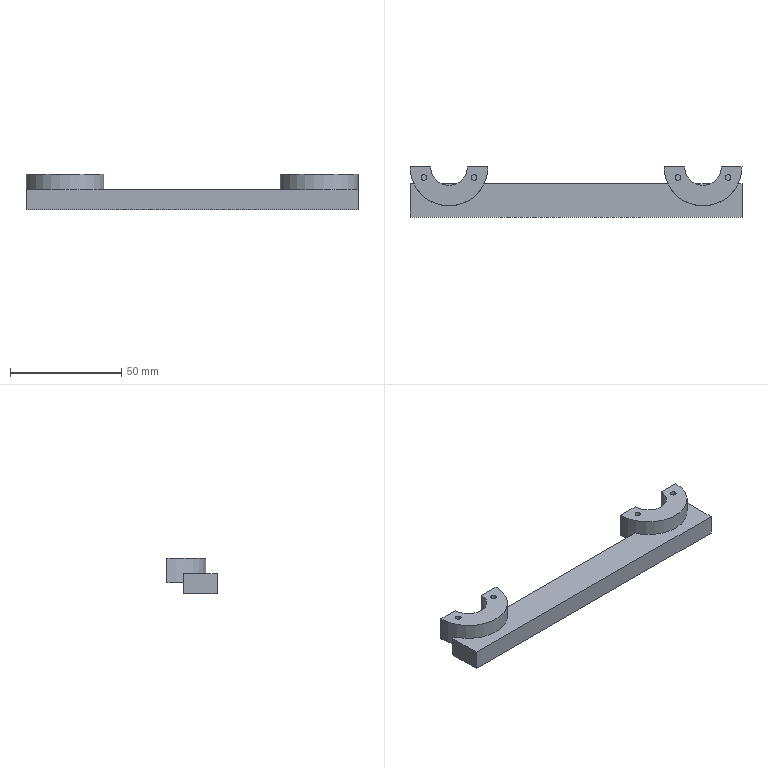Part | NX | 3 solids | 30 faces | box 149 x 22.5 x 16 mm | volume 26416 mm3 | plane 20 | cylinder 10 | commonest cylinder face diameters 2.5 x4 35 x4 16.5 x2
STEP:
#1=CARTESIAN_POINT('',(-53.811,-7.5,-7.));
#2=VERTEX_POINT('',#1);
#3=CARTESIAN_POINT('',(-22.189,-7.5,-7.));
#4=VERTEX_POINT('',#3);
#5=CARTESIAN_POINT('',(-38.,0.,-7.));
#6=DIRECTION('',(0.,0.,1.));
#7=DIRECTION('',(1.,0.,0.));
#8=AXIS2_PLACEMENT_3D('',#5,#6,#7);
#9=CIRCLE('',#8,17.5);
#10=EDGE_CURVE('',#2,#4,#9,.T.);
#11=ORIENTED_EDGE('',*,*,#10,.F.);
#12=CARTESIAN_POINT('',(-136.189,-7.5,-7.));
#13=VERTEX_POINT('',#12);
#14=CARTESIAN_POINT('',(-95.,-7.5,-7.));
#15=DIRECTION('',(1.,0.,0.));
#16=VECTOR('',#15,1000.);
#17=LINE('',#14,#16);
#18=EDGE_CURVE('',#13,#2,#17,.T.);
#19=ORIENTED_EDGE('',*,*,#18,.F.);
#20=CARTESIAN_POINT('',(-167.811,-7.5,-7.));
#21=VERTEX_POINT('',#20);
#22=CARTESIAN_POINT('',(-152.,0.,-7.));
#23=DIRECTION('',(0.,0.,1.));
#24=DIRECTION('',(1.,0.,0.));
#25=AXIS2_PLACEMENT_3D('',#22,#23,#24);
#26=CIRCLE('',#25,17.5);
#27=EDGE_CURVE('',#21,#13,#26,.T.);
#28=ORIENTED_EDGE('',*,*,#27,.F.);
#29=CARTESIAN_POINT('',(-169.5,-7.5,-7.));
#30=VERTEX_POINT('',#29);
#31=CARTESIAN_POINT('',(-95.,-7.5,-7.));
#32=DIRECTION('',(1.,0.,0.));
#33=VECTOR('',#32,1000.);
#34=LINE('',#31,#33);
#35=EDGE_CURVE('',#30,#21,#34,.T.);
#36=ORIENTED_EDGE('',*,*,#35,.F.);
#37=CARTESIAN_POINT('',(-169.5,-22.5,-7.));
#38=VERTEX_POINT('',#37);
#39=CARTESIAN_POINT('',(-169.5,-8.75,-7.));
#40=DIRECTION('',(0.,1.,0.));
#41=VECTOR('',#40,1000.);
#42=LINE('',#39,#41);
#43=EDGE_CURVE('',#38,#30,#42,.T.);
#44=ORIENTED_EDGE('',*,*,#43,.F.);
#45=CARTESIAN_POINT('',(-20.5,-22.5,-7.));
#46=VERTEX_POINT('',#45);
#47=CARTESIAN_POINT('',(-95.,-22.5,-7.));
#48=DIRECTION('',(-1.,0.,0.));
#49=VECTOR('',#48,1000.);
#50=LINE('',#47,#49);
#51=EDGE_CURVE('',#46,#38,#50,.T.);
#52=ORIENTED_EDGE('',*,*,#51,.F.);
#53=CARTESIAN_POINT('',(-20.5,-7.5,-7.));
#54=VERTEX_POINT('',#53);
#55=CARTESIAN_POINT('',(-20.5,-8.75,-7.));
#56=DIRECTION('',(0.,-1.,0.));
#57=VECTOR('',#56,1000.);
#58=LINE('',#55,#57);
#59=EDGE_CURVE('',#54,#46,#58,.T.);
#60=ORIENTED_EDGE('',*,*,#59,.F.);
#61=CARTESIAN_POINT('',(-95.,-7.5,-7.));
#62=DIRECTION('',(1.,0.,0.));
#63=VECTOR('',#62,1000.);
#64=LINE('',#61,#63);
#65=EDGE_CURVE('',#4,#54,#64,.T.);
#66=ORIENTED_EDGE('',*,*,#65,.F.);
#67=EDGE_LOOP('',(#11,#19,#28,#36,#44,#52,#60,#66));
#68=FACE_BOUND('',#67,.T.);
#69=CARTESIAN_POINT('',(-95.,-8.75,-7.));
#70=DIRECTION('',(0.,0.,1.));
#71=DIRECTION('',(1.,0.,0.));
#72=AXIS2_PLACEMENT_3D('',#69,#70,#71);
#73=PLANE('',#72);
#74=ADVANCED_FACE('',(#68),#73,.T.);
#75=CARTESIAN_POINT('',(-53.811,-7.5,-11.));
#76=VERTEX_POINT('',#75);
#77=CARTESIAN_POINT('',(-22.189,-7.5,-11.));
#78=VERTEX_POINT('',#77);
#79=CARTESIAN_POINT('',(-95.,-7.5,-11.));
#80=DIRECTION('',(1.,0.,0.));
#81=VECTOR('',#80,1000.);
#82=LINE('',#79,#81);
#83=EDGE_CURVE('',#76,#78,#82,.T.);
#84=ORIENTED_EDGE('',*,*,#83,.F.);
#85=CARTESIAN_POINT('',(-38.,0.,-11.));
#86=DIRECTION('',(0.,0.,1.));
#87=DIRECTION('',(1.,0.,0.));
#88=AXIS2_PLACEMENT_3D('',#85,#86,#87);
#89=CIRCLE('',#88,17.5);
#90=EDGE_CURVE('',#78,#76,#89,.F.);
#91=ORIENTED_EDGE('',*,*,#90,.F.);
#92=EDGE_LOOP('',(#84,#91));
#93=FACE_BOUND('',#92,.T.);
#94=CARTESIAN_POINT('',(-38.,0.,-11.));
#95=DIRECTION('',(0.,0.,1.));
#96=DIRECTION('',(1.,0.,0.));
#97=AXIS2_PLACEMENT_3D('',#94,#95,#96);
#98=PLANE('',#97);
#99=ADVANCED_FACE('',(#93),#98,.T.);
#100=CARTESIAN_POINT('',(-167.811,-7.5,-11.));
#101=VERTEX_POINT('',#100);
#102=CARTESIAN_POINT('',(-136.189,-7.5,-11.));
#103=VERTEX_POINT('',#102);
#104=CARTESIAN_POINT('',(-95.,-7.5,-11.));
#105=DIRECTION('',(1.,0.,0.));
#106=VECTOR('',#105,1000.);
#107=LINE('',#104,#106);
#108=EDGE_CURVE('',#101,#103,#107,.T.);
#109=ORIENTED_EDGE('',*,*,#108,.F.);
#110=CARTESIAN_POINT('',(-152.,0.,-11.));
#111=DIRECTION('',(0.,0.,1.));
#112=DIRECTION('',(1.,0.,0.));
#113=AXIS2_PLACEMENT_3D('',#110,#111,#112);
#114=CIRCLE('',#113,17.5);
#115=EDGE_CURVE('',#103,#101,#114,.F.);
#116=ORIENTED_EDGE('',*,*,#115,.F.);
#117=EDGE_LOOP('',(#109,#116));
#118=FACE_BOUND('',#117,.T.);
#119=CARTESIAN_POINT('',(-152.,0.,-11.));
#120=DIRECTION('',(0.,0.,1.));
#121=DIRECTION('',(1.,0.,0.));
#122=AXIS2_PLACEMENT_3D('',#119,#120,#121);
#123=PLANE('',#122);
#124=ADVANCED_FACE('',(#118),#123,.T.);
#125=CARTESIAN_POINT('',(-20.5,-22.5,-16.));
#126=VERTEX_POINT('',#125);
#127=CARTESIAN_POINT('',(-20.5,-22.5,-11.));
#128=DIRECTION('',(0.,0.,1.));
#129=VECTOR('',#128,1000.);
#130=LINE('',#127,#129);
#131=EDGE_CURVE('',#126,#46,#130,.T.);
#132=ORIENTED_EDGE('',*,*,#131,.T.);
#133=ORIENTED_EDGE('',*,*,#51,.T.);
#134=CARTESIAN_POINT('',(-169.5,-22.5,-16.));
#135=VERTEX_POINT('',#134);
#136=CARTESIAN_POINT('',(-169.5,-22.5,-11.));
#137=DIRECTION('',(0.,0.,1.));
#138=VECTOR('',#137,1000.);
#139=LINE('',#136,#138);
#140=EDGE_CURVE('',#135,#38,#139,.T.);
#141=ORIENTED_EDGE('',*,*,#140,.F.);
#142=CARTESIAN_POINT('',(-95.,-22.5,-16.));
#143=DIRECTION('',(1.,0.,0.));
#144=VECTOR('',#143,1000.);
#145=LINE('',#142,#144);
#146=EDGE_CURVE('',#135,#126,#145,.T.);
#147=ORIENTED_EDGE('',*,*,#146,.T.);
#148=EDGE_LOOP('',(#132,#133,#141,#147));
#149=FACE_BOUND('',#148,.T.);
#150=CARTESIAN_POINT('',(-95.,-22.5,-11.));
#151=DIRECTION('',(0.,-1.,0.));
#152=DIRECTION('',(0.,0.,-1.));
#153=AXIS2_PLACEMENT_3D('',#150,#151,#152);
#154=PLANE('',#153);
#155=ADVANCED_FACE('',(#149),#154,.T.);
#156=ORIENTED_EDGE('',*,*,#140,.T.);
#157=ORIENTED_EDGE('',*,*,#43,.T.);
#158=CARTESIAN_POINT('',(-169.5,-7.5,-16.));
#159=VERTEX_POINT('',#158);
#160=CARTESIAN_POINT('',(-169.5,-7.5,-11.));
#161=DIRECTION('',(0.,0.,1.));
#162=VECTOR('',#161,1000.);
#163=LINE('',#160,#162);
#164=EDGE_CURVE('',#159,#30,#163,.T.);
#165=ORIENTED_EDGE('',*,*,#164,.F.);
#166=CARTESIAN_POINT('',(-169.5,-8.75,-16.));
#167=DIRECTION('',(0.,-1.,0.));
#168=VECTOR('',#167,1000.);
#169=LINE('',#166,#168);
#170=EDGE_CURVE('',#159,#135,#169,.T.);
#171=ORIENTED_EDGE('',*,*,#170,.T.);
#172=EDGE_LOOP('',(#156,#157,#165,#171));
#173=FACE_BOUND('',#172,.T.);
#174=CARTESIAN_POINT('',(-169.5,-8.75,-11.));
#175=DIRECTION('',(-1.,0.,0.));
#176=DIRECTION('',(0.,0.,1.));
#177=AXIS2_PLACEMENT_3D('',#174,#175,#176);
#178=PLANE('',#177);
#179=ADVANCED_FACE('',(#173),#178,.T.);
#180=CARTESIAN_POINT('',(-53.811,-7.5,-11.));
#181=DIRECTION('',(0.,0.,1.));
#182=VECTOR('',#181,1000.);
#183=LINE('',#180,#182);
#184=EDGE_CURVE('',#76,#2,#183,.T.);
#185=ORIENTED_EDGE('',*,*,#184,.F.);
#186=ORIENTED_EDGE('',*,*,#83,.T.);
#187=CARTESIAN_POINT('',(-22.189,-7.5,-11.));
#188=DIRECTION('',(0.,0.,1.));
#189=VECTOR('',#188,1000.);
#190=LINE('',#187,#189);
#191=EDGE_CURVE('',#4,#78,#190,.F.);
#192=ORIENTED_EDGE('',*,*,#191,.F.);
#193=ORIENTED_EDGE('',*,*,#65,.T.);
#194=CARTESIAN_POINT('',(-20.5,-7.5,-16.));
#195=VERTEX_POINT('',#194);
#196=CARTESIAN_POINT('',(-20.5,-7.5,-11.));
#197=DIRECTION('',(0.,0.,1.));
#198=VECTOR('',#197,1000.);
#199=LINE('',#196,#198);
#200=EDGE_CURVE('',#195,#54,#199,.T.);
#201=ORIENTED_EDGE('',*,*,#200,.F.);
#202=CARTESIAN_POINT('',(-95.,-7.5,-16.));
#203=DIRECTION('',(-1.,0.,0.));
#204=VECTOR('',#203,1000.);
#205=LINE('',#202,#204);
#206=EDGE_CURVE('',#195,#159,#205,.T.);
#207=ORIENTED_EDGE('',*,*,#206,.T.);
#208=ORIENTED_EDGE('',*,*,#164,.T.);
#209=ORIENTED_EDGE('',*,*,#35,.T.);
#210=CARTESIAN_POINT('',(-167.811,-7.5,-11.));
#211=DIRECTION('',(0.,0.,1.));
#212=VECTOR('',#211,1000.);
#213=LINE('',#210,#212);
#214=EDGE_CURVE('',#101,#21,#213,.T.);
#215=ORIENTED_EDGE('',*,*,#214,.F.);
#216=ORIENTED_EDGE('',*,*,#108,.T.);
#217=CARTESIAN_POINT('',(-136.189,-7.5,-11.));
#218=DIRECTION('',(0.,0.,1.));
#219=VECTOR('',#218,1000.);
#220=LINE('',#217,#219);
#221=EDGE_CURVE('',#13,#103,#220,.F.);
#222=ORIENTED_EDGE('',*,*,#221,.F.);
#223=ORIENTED_EDGE('',*,*,#18,.T.);
#224=EDGE_LOOP('',(#185,#186,#192,#193,#201,#207,#208,#209,#215,#216,#222,#223));
#225=FACE_BOUND('',#224,.T.);
#226=CARTESIAN_POINT('',(-95.,-7.5,-11.));
#227=DIRECTION('',(0.,1.,0.));
#228=DIRECTION('',(0.,0.,1.));
#229=AXIS2_PLACEMENT_3D('',#226,#227,#228);
#230=PLANE('',#229);
#231=ADVANCED_FACE('',(#225),#230,.T.);
#232=CARTESIAN_POINT('',(-20.5,-8.75,-16.));
#233=DIRECTION('',(0.,1.,0.));
#234=VECTOR('',#233,1000.);
#235=LINE('',#232,#234);
#236=EDGE_CURVE('',#126,#195,#235,.T.);
#237=ORIENTED_EDGE('',*,*,#236,.F.);
#238=ORIENTED_EDGE('',*,*,#146,.F.);
#239=ORIENTED_EDGE('',*,*,#170,.F.);
#240=ORIENTED_EDGE('',*,*,#206,.F.);
#241=EDGE_LOOP('',(#237,#238,#239,#240));
#242=FACE_BOUND('',#241,.T.);
#243=CARTESIAN_POINT('',(-95.,-8.75,-16.));
#244=DIRECTION('',(0.,0.,-1.));
#245=DIRECTION('',(-1.,0.,0.));
#246=AXIS2_PLACEMENT_3D('',#243,#244,#245);
#247=PLANE('',#246);
#248=ADVANCED_FACE('',(#242),#247,.T.);
#249=ORIENTED_EDGE('',*,*,#236,.T.);
#250=ORIENTED_EDGE('',*,*,#200,.T.);
#251=ORIENTED_EDGE('',*,*,#59,.T.);
#252=ORIENTED_EDGE('',*,*,#131,.F.);
#253=EDGE_LOOP('',(#249,#250,#251,#252));
#254=FACE_BOUND('',#253,.T.);
#255=CARTESIAN_POINT('',(-20.5,-8.75,-11.));
#256=DIRECTION('',(1.,0.,0.));
#257=DIRECTION('',(0.,0.,-1.));
#258=AXIS2_PLACEMENT_3D('',#255,#256,#257);
#259=PLANE('',#258);
#260=ADVANCED_FACE('',(#254),#259,.T.);
#261=ORIENTED_EDGE('',*,*,#214,.T.);
#262=ORIENTED_EDGE('',*,*,#27,.T.);
#263=ORIENTED_EDGE('',*,*,#221,.T.);
#264=ORIENTED_EDGE('',*,*,#115,.T.);
#265=EDGE_LOOP('',(#261,#262,#263,#264));
#266=FACE_BOUND('',#265,.T.);
#267=CARTESIAN_POINT('',(-152.,0.,-11.));
#268=DIRECTION('',(0.,0.,1.));
#269=DIRECTION('',(1.,0.,0.));
#270=AXIS2_PLACEMENT_3D('',#267,#268,#269);
#271=CYLINDRICAL_SURFACE('',#270,17.5);
#272=ADVANCED_FACE('',(#266),#271,.F.);
#273=ORIENTED_EDGE('',*,*,#184,.T.);
#274=ORIENTED_EDGE('',*,*,#10,.T.);
#275=ORIENTED_EDGE('',*,*,#191,.T.);
#276=ORIENTED_EDGE('',*,*,#90,.T.);
#277=EDGE_LOOP('',(#273,#274,#275,#276));
#278=FACE_BOUND('',#277,.T.);
#279=CARTESIAN_POINT('',(-38.,0.,-11.));
#280=DIRECTION('',(0.,0.,1.));
#281=DIRECTION('',(1.,0.,0.));
#282=AXIS2_PLACEMENT_3D('',#279,#280,#281);
#283=CYLINDRICAL_SURFACE('',#282,17.5);
#284=ADVANCED_FACE('',(#278),#283,.F.);
#285=CLOSED_SHELL('',(#74,#99,#124,#155,#179,#231,#248,#260,#272,#284));
#286=MANIFOLD_SOLID_BREP('',#285);
#287=CARTESIAN_POINT('',(-160.25,0.,0.));
#288=VERTEX_POINT('',#287);
#289=CARTESIAN_POINT('',(-169.5,0.,0.));
#290=VERTEX_POINT('',#289);
#291=CARTESIAN_POINT('',(-160.25,0.,0.));
#292=DIRECTION('',(-1.,0.,0.));
#293=VECTOR('',#292,1000.);
#294=LINE('',#291,#293);
#295=EDGE_CURVE('',#288,#290,#294,.T.);
#296=ORIENTED_EDGE('',*,*,#295,.F.);
#297=CARTESIAN_POINT('',(-160.25,0.,-11.));
#298=VERTEX_POINT('',#297);
#299=CARTESIAN_POINT('',(-160.25,0.,-11.));
#300=DIRECTION('',(0.,0.,1.));
#301=VECTOR('',#300,1000.);
#302=LINE('',#299,#301);
#303=EDGE_CURVE('',#298,#288,#302,.T.);
#304=ORIENTED_EDGE('',*,*,#303,.F.);
#305=CARTESIAN_POINT('',(-169.5,0.,-11.));
#306=VERTEX_POINT('',#305);
#307=CARTESIAN_POINT('',(-160.25,0.,-11.));
#308=DIRECTION('',(-1.,0.,0.));
#309=VECTOR('',#308,1000.);
#310=LINE('',#307,#309);
#311=EDGE_CURVE('',#298,#306,#310,.T.);
#312=ORIENTED_EDGE('',*,*,#311,.T.);
#313=CARTESIAN_POINT('',(-169.5,0.,-11.));
#314=DIRECTION('',(0.,0.,1.));
#315=VECTOR('',#314,1000.);
#316=LINE('',#313,#315);
#317=EDGE_CURVE('',#306,#290,#316,.T.);
#318=ORIENTED_EDGE('',*,*,#317,.T.);
#319=EDGE_LOOP('',(#296,#304,#312,#318));
#320=FACE_BOUND('',#319,.T.);
#321=CARTESIAN_POINT('',(-160.25,0.,-11.));
#322=DIRECTION('',(0.,1.,0.));
#323=DIRECTION('',(-1.,0.,0.));
#324=AXIS2_PLACEMENT_3D('',#321,#322,#323);
#325=PLANE('',#324);
#326=ADVANCED_FACE('',(#320),#325,.T.);
#327=CARTESIAN_POINT('',(-134.5,0.,0.));
#328=VERTEX_POINT('',#327);
#329=CARTESIAN_POINT('',(-152.,0.,0.));
#330=DIRECTION('',(0.,0.,1.));
#331=DIRECTION('',(1.,0.,0.));
#332=AXIS2_PLACEMENT_3D('',#329,#330,#331);
#333=CIRCLE('',#332,17.5);
#334=EDGE_CURVE('',#290,#328,#333,.T.);
#335=ORIENTED_EDGE('',*,*,#334,.F.);
#336=ORIENTED_EDGE('',*,*,#317,.F.);
#337=CARTESIAN_POINT('',(-134.5,0.,-11.));
#338=VERTEX_POINT('',#337);
#339=CARTESIAN_POINT('',(-152.,0.,-11.));
#340=DIRECTION('',(0.,0.,1.));
#341=DIRECTION('',(1.,0.,0.));
#342=AXIS2_PLACEMENT_3D('',#339,#340,#341);
#343=CIRCLE('',#342,17.5);
#344=EDGE_CURVE('',#306,#338,#343,.T.);
#345=ORIENTED_EDGE('',*,*,#344,.T.);
#346=CARTESIAN_POINT('',(-134.5,0.,-11.));
#347=DIRECTION('',(0.,0.,1.));
#348=VECTOR('',#347,1000.);
#349=LINE('',#346,#348);
#350=EDGE_CURVE('',#338,#328,#349,.T.);
#351=ORIENTED_EDGE('',*,*,#350,.T.);
#352=EDGE_LOOP('',(#335,#336,#345,#351));
#353=FACE_BOUND('',#352,.T.);
#354=CARTESIAN_POINT('',(-152.,0.,-11.));
#355=DIRECTION('',(0.,0.,1.));
#356=DIRECTION('',(1.,0.,0.));
#357=AXIS2_PLACEMENT_3D('',#354,#355,#356);
#358=CYLINDRICAL_SURFACE('',#357,17.5);
#359=ADVANCED_FACE('',(#353),#358,.T.);
#360=CARTESIAN_POINT('',(-143.75,0.,0.));
#361=VERTEX_POINT('',#360);
#362=CARTESIAN_POINT('',(-134.5,0.,0.));
#363=DIRECTION('',(-1.,0.,0.));
#364=VECTOR('',#363,1000.);
#365=LINE('',#362,#364);
#366=EDGE_CURVE('',#328,#361,#365,.T.);
#367=ORIENTED_EDGE('',*,*,#366,.F.);
#368=ORIENTED_EDGE('',*,*,#350,.F.);
#369=CARTESIAN_POINT('',(-143.75,0.,-11.));
#370=VERTEX_POINT('',#369);
#371=CARTESIAN_POINT('',(-134.5,0.,-11.));
#372=DIRECTION('',(-1.,0.,0.));
#373=VECTOR('',#372,1000.);
#374=LINE('',#371,#373);
#375=EDGE_CURVE('',#338,#370,#374,.T.);
#376=ORIENTED_EDGE('',*,*,#375,.T.);
#377=CARTESIAN_POINT('',(-143.75,0.,-11.));
#378=DIRECTION('',(0.,0.,1.));
#379=VECTOR('',#378,1000.);
#380=LINE('',#377,#379);
#381=EDGE_CURVE('',#370,#361,#380,.T.);
#382=ORIENTED_EDGE('',*,*,#381,.T.);
#383=EDGE_LOOP('',(#367,#368,#376,#382));
#384=FACE_BOUND('',#383,.T.);
#385=CARTESIAN_POINT('',(-134.5,0.,-11.));
#386=DIRECTION('',(0.,1.,0.));
#387=DIRECTION('',(-1.,0.,0.));
#388=AXIS2_PLACEMENT_3D('',#385,#386,#387);
#389=PLANE('',#388);
#390=ADVANCED_FACE('',(#384),#389,.T.);
#391=CARTESIAN_POINT('',(-152.,0.,0.));
#392=DIRECTION('',(0.,0.,-1.));
#393=DIRECTION('',(1.,0.,0.));
#394=AXIS2_PLACEMENT_3D('',#391,#392,#393);
#395=CIRCLE('',#394,8.25);
#396=EDGE_CURVE('',#361,#288,#395,.T.);
#397=ORIENTED_EDGE('',*,*,#396,.F.);
#398=ORIENTED_EDGE('',*,*,#381,.F.);
#399=CARTESIAN_POINT('',(-152.,0.,-11.));
#400=DIRECTION('',(0.,0.,-1.));
#401=DIRECTION('',(1.,0.,0.));
#402=AXIS2_PLACEMENT_3D('',#399,#400,#401);
#403=CIRCLE('',#402,8.25);
#404=EDGE_CURVE('',#370,#298,#403,.T.);
#405=ORIENTED_EDGE('',*,*,#404,.T.);
#406=ORIENTED_EDGE('',*,*,#303,.T.);
#407=EDGE_LOOP('',(#397,#398,#405,#406));
#408=FACE_BOUND('',#407,.T.);
#409=CARTESIAN_POINT('',(-152.,0.,-11.));
#410=DIRECTION('',(0.,0.,1.));
#411=DIRECTION('',(1.,0.,0.));
#412=AXIS2_PLACEMENT_3D('',#409,#410,#411);
#413=CYLINDRICAL_SURFACE('',#412,8.25);
#414=ADVANCED_FACE('',(#408),#413,.F.);
#415=ORIENTED_EDGE('',*,*,#311,.F.);
#416=ORIENTED_EDGE('',*,*,#404,.F.);
#417=ORIENTED_EDGE('',*,*,#375,.F.);
#418=ORIENTED_EDGE('',*,*,#344,.F.);
#419=EDGE_LOOP('',(#415,#416,#417,#418));
#420=FACE_BOUND('',#419,.T.);
#421=CARTESIAN_POINT('',(-152.,0.,-11.));
#422=DIRECTION('',(0.,0.,1.));
#423=DIRECTION('',(1.,0.,0.));
#424=AXIS2_PLACEMENT_3D('',#421,#422,#423);
#425=PLANE('',#424);
#426=ADVANCED_FACE('',(#420),#425,.F.);
#427=CARTESIAN_POINT('',(-139.5,-4.75,0.));
#428=VERTEX_POINT('',#427);
#429=CARTESIAN_POINT('',(-140.75,-4.75,0.));
#430=DIRECTION('',(0.,0.,1.));
#431=DIRECTION('',(1.,0.,0.));
#432=AXIS2_PLACEMENT_3D('',#429,#430,#431);
#433=CIRCLE('',#432,1.25);
#434=EDGE_CURVE('',#428,#428,#433,.T.);
#435=ORIENTED_EDGE('',*,*,#434,.F.);
#436=EDGE_LOOP('',(#435));
#437=FACE_BOUND('',#436,.T.);
#438=CARTESIAN_POINT('',(-162.,-4.75,0.));
#439=VERTEX_POINT('',#438);
#440=CARTESIAN_POINT('',(-163.25,-4.75,0.));
#441=DIRECTION('',(0.,0.,1.));
#442=DIRECTION('',(1.,0.,0.));
#443=AXIS2_PLACEMENT_3D('',#440,#441,#442);
#444=CIRCLE('',#443,1.25);
#445=EDGE_CURVE('',#439,#439,#444,.T.);
#446=ORIENTED_EDGE('',*,*,#445,.F.);
#447=EDGE_LOOP('',(#446));
#448=FACE_BOUND('',#447,.T.);
#449=ORIENTED_EDGE('',*,*,#295,.T.);
#450=ORIENTED_EDGE('',*,*,#334,.T.);
#451=ORIENTED_EDGE('',*,*,#366,.T.);
#452=ORIENTED_EDGE('',*,*,#396,.T.);
#453=EDGE_LOOP('',(#449,#450,#451,#452));
#454=FACE_BOUND('',#453,.T.);
#455=CARTESIAN_POINT('',(-152.,0.,0.));
#456=DIRECTION('',(0.,0.,1.));
#457=DIRECTION('',(1.,0.,0.));
#458=AXIS2_PLACEMENT_3D('',#455,#456,#457);
#459=PLANE('',#458);
#460=ADVANCED_FACE('',(#437,#448,#454),#459,.T.);
#461=CARTESIAN_POINT('',(-162.,-4.75,-5.9));
#462=VERTEX_POINT('',#461);
#463=CARTESIAN_POINT('',(-163.25,-4.75,-5.9));
#464=DIRECTION('',(0.,0.,1.));
#465=DIRECTION('',(1.,0.,0.));
#466=AXIS2_PLACEMENT_3D('',#463,#464,#465);
#467=CIRCLE('',#466,1.25);
#468=EDGE_CURVE('',#462,#462,#467,.F.);
#469=ORIENTED_EDGE('',*,*,#468,.T.);
#470=EDGE_LOOP('',(#469));
#471=FACE_BOUND('',#470,.T.);
#472=ORIENTED_EDGE('',*,*,#445,.T.);
#473=EDGE_LOOP('',(#472));
#474=FACE_BOUND('',#473,.T.);
#475=CARTESIAN_POINT('',(-163.25,-4.75,-5.9));
#476=DIRECTION('',(0.,0.,1.));
#477=DIRECTION('',(1.,0.,0.));
#478=AXIS2_PLACEMENT_3D('',#475,#476,#477);
#479=CYLINDRICAL_SURFACE('',#478,1.25);
#480=ADVANCED_FACE('',(#471,#474),#479,.F.);
#481=ORIENTED_EDGE('',*,*,#468,.F.);
#482=EDGE_LOOP('',(#481));
#483=FACE_BOUND('',#482,.T.);
#484=CARTESIAN_POINT('',(-163.25,-4.75,-5.9));
#485=DIRECTION('',(0.,0.,1.));
#486=DIRECTION('',(1.,0.,0.));
#487=AXIS2_PLACEMENT_3D('',#484,#485,#486);
#488=PLANE('',#487);
#489=ADVANCED_FACE('',(#483),#488,.T.);
#490=CARTESIAN_POINT('',(-139.5,-4.75,-5.9));
#491=VERTEX_POINT('',#490);
#492=CARTESIAN_POINT('',(-140.75,-4.75,-5.9));
#493=DIRECTION('',(0.,0.,1.));
#494=DIRECTION('',(1.,0.,0.));
#495=AXIS2_PLACEMENT_3D('',#492,#493,#494);
#496=CIRCLE('',#495,1.25);
#497=EDGE_CURVE('',#491,#491,#496,.F.);
#498=ORIENTED_EDGE('',*,*,#497,.T.);
#499=EDGE_LOOP('',(#498));
#500=FACE_BOUND('',#499,.T.);
#501=ORIENTED_EDGE('',*,*,#434,.T.);
#502=EDGE_LOOP('',(#501));
#503=FACE_BOUND('',#502,.T.);
#504=CARTESIAN_POINT('',(-140.75,-4.75,-5.9));
#505=DIRECTION('',(0.,0.,1.));
#506=DIRECTION('',(1.,0.,0.));
#507=AXIS2_PLACEMENT_3D('',#504,#505,#506);
#508=CYLINDRICAL_SURFACE('',#507,1.25);
#509=ADVANCED_FACE('',(#500,#503),#508,.F.);
#510=ORIENTED_EDGE('',*,*,#497,.F.);
#511=EDGE_LOOP('',(#510));
#512=FACE_BOUND('',#511,.T.);
#513=CARTESIAN_POINT('',(-140.75,-4.75,-5.9));
#514=DIRECTION('',(0.,0.,1.));
#515=DIRECTION('',(1.,0.,0.));
#516=AXIS2_PLACEMENT_3D('',#513,#514,#515);
#517=PLANE('',#516);
#518=ADVANCED_FACE('',(#512),#517,.T.);
#519=CLOSED_SHELL('',(#326,#359,#390,#414,#426,#460,#480,#489,#509,#518));
#520=MANIFOLD_SOLID_BREP('',#519);
#521=CARTESIAN_POINT('',(-46.25,0.,0.));
#522=VERTEX_POINT('',#521);
#523=CARTESIAN_POINT('',(-55.5,0.,0.));
#524=VERTEX_POINT('',#523);
#525=CARTESIAN_POINT('',(-46.25,0.,0.));
#526=DIRECTION('',(-1.,0.,0.));
#527=VECTOR('',#526,1000.);
#528=LINE('',#525,#527);
#529=EDGE_CURVE('',#522,#524,#528,.T.);
#530=ORIENTED_EDGE('',*,*,#529,.F.);
#531=CARTESIAN_POINT('',(-46.25,0.,-11.));
#532=VERTEX_POINT('',#531);
#533=CARTESIAN_POINT('',(-46.25,0.,-11.));
#534=DIRECTION('',(0.,0.,1.));
#535=VECTOR('',#534,1000.);
#536=LINE('',#533,#535);
#537=EDGE_CURVE('',#532,#522,#536,.T.);
#538=ORIENTED_EDGE('',*,*,#537,.F.);
#539=CARTESIAN_POINT('',(-55.5,0.,-11.));
#540=VERTEX_POINT('',#539);
#541=CARTESIAN_POINT('',(-46.25,0.,-11.));
#542=DIRECTION('',(-1.,0.,0.));
#543=VECTOR('',#542,1000.);
#544=LINE('',#541,#543);
#545=EDGE_CURVE('',#532,#540,#544,.T.);
#546=ORIENTED_EDGE('',*,*,#545,.T.);
#547=CARTESIAN_POINT('',(-55.5,0.,-11.));
#548=DIRECTION('',(0.,0.,1.));
#549=VECTOR('',#548,1000.);
#550=LINE('',#547,#549);
#551=EDGE_CURVE('',#540,#524,#550,.T.);
#552=ORIENTED_EDGE('',*,*,#551,.T.);
#553=EDGE_LOOP('',(#530,#538,#546,#552));
#554=FACE_BOUND('',#553,.T.);
#555=CARTESIAN_POINT('',(-46.25,0.,-11.));
#556=DIRECTION('',(0.,1.,0.));
#557=DIRECTION('',(-1.,0.,0.));
#558=AXIS2_PLACEMENT_3D('',#555,#556,#557);
#559=PLANE('',#558);
#560=ADVANCED_FACE('',(#554),#559,.T.);
#561=CARTESIAN_POINT('',(-20.5,0.,0.));
#562=VERTEX_POINT('',#561);
#563=CARTESIAN_POINT('',(-38.,0.,0.));
#564=DIRECTION('',(0.,0.,1.));
#565=DIRECTION('',(1.,0.,0.));
#566=AXIS2_PLACEMENT_3D('',#563,#564,#565);
#567=CIRCLE('',#566,17.5);
#568=EDGE_CURVE('',#524,#562,#567,.T.);
#569=ORIENTED_EDGE('',*,*,#568,.F.);
#570=ORIENTED_EDGE('',*,*,#551,.F.);
#571=CARTESIAN_POINT('',(-20.5,0.,-11.));
#572=VERTEX_POINT('',#571);
#573=CARTESIAN_POINT('',(-38.,0.,-11.));
#574=DIRECTION('',(0.,0.,1.));
#575=DIRECTION('',(1.,0.,0.));
#576=AXIS2_PLACEMENT_3D('',#573,#574,#575);
#577=CIRCLE('',#576,17.5);
#578=EDGE_CURVE('',#540,#572,#577,.T.);
#579=ORIENTED_EDGE('',*,*,#578,.T.);
#580=CARTESIAN_POINT('',(-20.5,0.,-11.));
#581=DIRECTION('',(0.,0.,1.));
#582=VECTOR('',#581,1000.);
#583=LINE('',#580,#582);
#584=EDGE_CURVE('',#572,#562,#583,.T.);
#585=ORIENTED_EDGE('',*,*,#584,.T.);
#586=EDGE_LOOP('',(#569,#570,#579,#585));
#587=FACE_BOUND('',#586,.T.);
#588=CARTESIAN_POINT('',(-38.,0.,-11.));
#589=DIRECTION('',(0.,0.,1.));
#590=DIRECTION('',(1.,0.,0.));
#591=AXIS2_PLACEMENT_3D('',#588,#589,#590);
#592=CYLINDRICAL_SURFACE('',#591,17.5);
#593=ADVANCED_FACE('',(#587),#592,.T.);
#594=CARTESIAN_POINT('',(-29.75,0.,0.));
#595=VERTEX_POINT('',#594);
#596=CARTESIAN_POINT('',(-20.5,0.,0.));
#597=DIRECTION('',(-1.,0.,0.));
#598=VECTOR('',#597,1000.);
#599=LINE('',#596,#598);
#600=EDGE_CURVE('',#562,#595,#599,.T.);
#601=ORIENTED_EDGE('',*,*,#600,.F.);
#602=ORIENTED_EDGE('',*,*,#584,.F.);
#603=CARTESIAN_POINT('',(-29.75,0.,-11.));
#604=VERTEX_POINT('',#603);
#605=CARTESIAN_POINT('',(-20.5,0.,-11.));
#606=DIRECTION('',(-1.,0.,0.));
#607=VECTOR('',#606,1000.);
#608=LINE('',#605,#607);
#609=EDGE_CURVE('',#572,#604,#608,.T.);
#610=ORIENTED_EDGE('',*,*,#609,.T.);
#611=CARTESIAN_POINT('',(-29.75,0.,-11.));
#612=DIRECTION('',(0.,0.,1.));
#613=VECTOR('',#612,1000.);
#614=LINE('',#611,#613);
#615=EDGE_CURVE('',#604,#595,#614,.T.);
#616=ORIENTED_EDGE('',*,*,#615,.T.);
#617=EDGE_LOOP('',(#601,#602,#610,#616));
#618=FACE_BOUND('',#617,.T.);
#619=CARTESIAN_POINT('',(-20.5,0.,-11.));
#620=DIRECTION('',(0.,1.,0.));
#621=DIRECTION('',(-1.,0.,0.));
#622=AXIS2_PLACEMENT_3D('',#619,#620,#621);
#623=PLANE('',#622);
#624=ADVANCED_FACE('',(#618),#623,.T.);
#625=CARTESIAN_POINT('',(-38.,0.,0.));
#626=DIRECTION('',(0.,0.,-1.));
#627=DIRECTION('',(1.,0.,0.));
#628=AXIS2_PLACEMENT_3D('',#625,#626,#627);
#629=CIRCLE('',#628,8.25);
#630=EDGE_CURVE('',#595,#522,#629,.T.);
#631=ORIENTED_EDGE('',*,*,#630,.F.);
#632=ORIENTED_EDGE('',*,*,#615,.F.);
#633=CARTESIAN_POINT('',(-38.,0.,-11.));
#634=DIRECTION('',(0.,0.,-1.));
#635=DIRECTION('',(1.,0.,0.));
#636=AXIS2_PLACEMENT_3D('',#633,#634,#635);
#637=CIRCLE('',#636,8.25);
#638=EDGE_CURVE('',#604,#532,#637,.T.);
#639=ORIENTED_EDGE('',*,*,#638,.T.);
#640=ORIENTED_EDGE('',*,*,#537,.T.);
#641=EDGE_LOOP('',(#631,#632,#639,#640));
#642=FACE_BOUND('',#641,.T.);
#643=CARTESIAN_POINT('',(-38.,0.,-11.));
#644=DIRECTION('',(0.,0.,1.));
#645=DIRECTION('',(1.,0.,0.));
#646=AXIS2_PLACEMENT_3D('',#643,#644,#645);
#647=CYLINDRICAL_SURFACE('',#646,8.25);
#648=ADVANCED_FACE('',(#642),#647,.F.);
#649=ORIENTED_EDGE('',*,*,#545,.F.);
#650=ORIENTED_EDGE('',*,*,#638,.F.);
#651=ORIENTED_EDGE('',*,*,#609,.F.);
#652=ORIENTED_EDGE('',*,*,#578,.F.);
#653=EDGE_LOOP('',(#649,#650,#651,#652));
#654=FACE_BOUND('',#653,.T.);
#655=CARTESIAN_POINT('',(-38.,0.,-11.));
#656=DIRECTION('',(0.,0.,1.));
#657=DIRECTION('',(1.,0.,0.));
#658=AXIS2_PLACEMENT_3D('',#655,#656,#657);
#659=PLANE('',#658);
#660=ADVANCED_FACE('',(#654),#659,.F.);
#661=CARTESIAN_POINT('',(-25.5,-4.75,0.));
#662=VERTEX_POINT('',#661);
#663=CARTESIAN_POINT('',(-26.75,-4.75,0.));
#664=DIRECTION('',(0.,0.,1.));
#665=DIRECTION('',(1.,0.,0.));
#666=AXIS2_PLACEMENT_3D('',#663,#664,#665);
#667=CIRCLE('',#666,1.25);
#668=EDGE_CURVE('',#662,#662,#667,.T.);
#669=ORIENTED_EDGE('',*,*,#668,.F.);
#670=EDGE_LOOP('',(#669));
#671=FACE_BOUND('',#670,.T.);
#672=CARTESIAN_POINT('',(-48.,-4.75,0.));
#673=VERTEX_POINT('',#672);
#674=CARTESIAN_POINT('',(-49.25,-4.75,0.));
#675=DIRECTION('',(0.,0.,1.));
#676=DIRECTION('',(1.,0.,0.));
#677=AXIS2_PLACEMENT_3D('',#674,#675,#676);
#678=CIRCLE('',#677,1.25);
#679=EDGE_CURVE('',#673,#673,#678,.T.);
#680=ORIENTED_EDGE('',*,*,#679,.F.);
#681=EDGE_LOOP('',(#680));
#682=FACE_BOUND('',#681,.T.);
#683=ORIENTED_EDGE('',*,*,#529,.T.);
#684=ORIENTED_EDGE('',*,*,#568,.T.);
#685=ORIENTED_EDGE('',*,*,#600,.T.);
#686=ORIENTED_EDGE('',*,*,#630,.T.);
#687=EDGE_LOOP('',(#683,#684,#685,#686));
#688=FACE_BOUND('',#687,.T.);
#689=CARTESIAN_POINT('',(-38.,0.,0.));
#690=DIRECTION('',(0.,0.,1.));
#691=DIRECTION('',(1.,0.,0.));
#692=AXIS2_PLACEMENT_3D('',#689,#690,#691);
#693=PLANE('',#692);
#694=ADVANCED_FACE('',(#671,#682,#688),#693,.T.);
#695=CARTESIAN_POINT('',(-48.,-4.75,-5.9));
#696=VERTEX_POINT('',#695);
#697=CARTESIAN_POINT('',(-49.25,-4.75,-5.9));
#698=DIRECTION('',(0.,0.,1.));
#699=DIRECTION('',(1.,0.,0.));
#700=AXIS2_PLACEMENT_3D('',#697,#698,#699);
#701=CIRCLE('',#700,1.25);
#702=EDGE_CURVE('',#696,#696,#701,.F.);
#703=ORIENTED_EDGE('',*,*,#702,.T.);
#704=EDGE_LOOP('',(#703));
#705=FACE_BOUND('',#704,.T.);
#706=ORIENTED_EDGE('',*,*,#679,.T.);
#707=EDGE_LOOP('',(#706));
#708=FACE_BOUND('',#707,.T.);
#709=CARTESIAN_POINT('',(-49.25,-4.75,-5.9));
#710=DIRECTION('',(0.,0.,1.));
#711=DIRECTION('',(1.,0.,0.));
#712=AXIS2_PLACEMENT_3D('',#709,#710,#711);
#713=CYLINDRICAL_SURFACE('',#712,1.25);
#714=ADVANCED_FACE('',(#705,#708),#713,.F.);
#715=ORIENTED_EDGE('',*,*,#702,.F.);
#716=EDGE_LOOP('',(#715));
#717=FACE_BOUND('',#716,.T.);
#718=CARTESIAN_POINT('',(-49.25,-4.75,-5.9));
#719=DIRECTION('',(0.,0.,1.));
#720=DIRECTION('',(1.,0.,0.));
#721=AXIS2_PLACEMENT_3D('',#718,#719,#720);
#722=PLANE('',#721);
#723=ADVANCED_FACE('',(#717),#722,.T.);
#724=CARTESIAN_POINT('',(-25.5,-4.75,-5.9));
#725=VERTEX_POINT('',#724);
#726=CARTESIAN_POINT('',(-26.75,-4.75,-5.9));
#727=DIRECTION('',(0.,0.,1.));
#728=DIRECTION('',(1.,0.,0.));
#729=AXIS2_PLACEMENT_3D('',#726,#727,#728);
#730=CIRCLE('',#729,1.25);
#731=EDGE_CURVE('',#725,#725,#730,.F.);
#732=ORIENTED_EDGE('',*,*,#731,.T.);
#733=EDGE_LOOP('',(#732));
#734=FACE_BOUND('',#733,.T.);
#735=ORIENTED_EDGE('',*,*,#668,.T.);
#736=EDGE_LOOP('',(#735));
#737=FACE_BOUND('',#736,.T.);
#738=CARTESIAN_POINT('',(-26.75,-4.75,-5.9));
#739=DIRECTION('',(0.,0.,1.));
#740=DIRECTION('',(1.,0.,0.));
#741=AXIS2_PLACEMENT_3D('',#738,#739,#740);
#742=CYLINDRICAL_SURFACE('',#741,1.25);
#743=ADVANCED_FACE('',(#734,#737),#742,.F.);
#744=ORIENTED_EDGE('',*,*,#731,.F.);
#745=EDGE_LOOP('',(#744));
#746=FACE_BOUND('',#745,.T.);
#747=CARTESIAN_POINT('',(-26.75,-4.75,-5.9));
#748=DIRECTION('',(0.,0.,1.));
#749=DIRECTION('',(1.,0.,0.));
#750=AXIS2_PLACEMENT_3D('',#747,#748,#749);
#751=PLANE('',#750);
#752=ADVANCED_FACE('',(#746),#751,.T.);
#753=CLOSED_SHELL('',(#560,#593,#624,#648,#660,#694,#714,#723,#743,#752));
#754=MANIFOLD_SOLID_BREP('',#753);
#755=(LENGTH_UNIT()NAMED_UNIT(*)SI_UNIT(.MILLI.,.METRE.));
#756=UNCERTAINTY_MEASURE_WITH_UNIT(LENGTH_MEASURE(0.00001),#755,'','');
#757=(NAMED_UNIT(*)PLANE_ANGLE_UNIT()SI_UNIT($,.RADIAN.));
#758=(NAMED_UNIT(*)SI_UNIT($,.STERADIAN.)SOLID_ANGLE_UNIT());
#759=(GEOMETRIC_REPRESENTATION_CONTEXT(3)GLOBAL_UNCERTAINTY_ASSIGNED_CONTEXT((#756))GLOBAL_UNIT_ASSIGNED_CONTEXT((#755,#757,#758))REPRESENTATION_CONTEXT('',''));
#760=ADVANCED_BREP_SHAPE_REPRESENTATION('',(#286,#520,#754),#759);